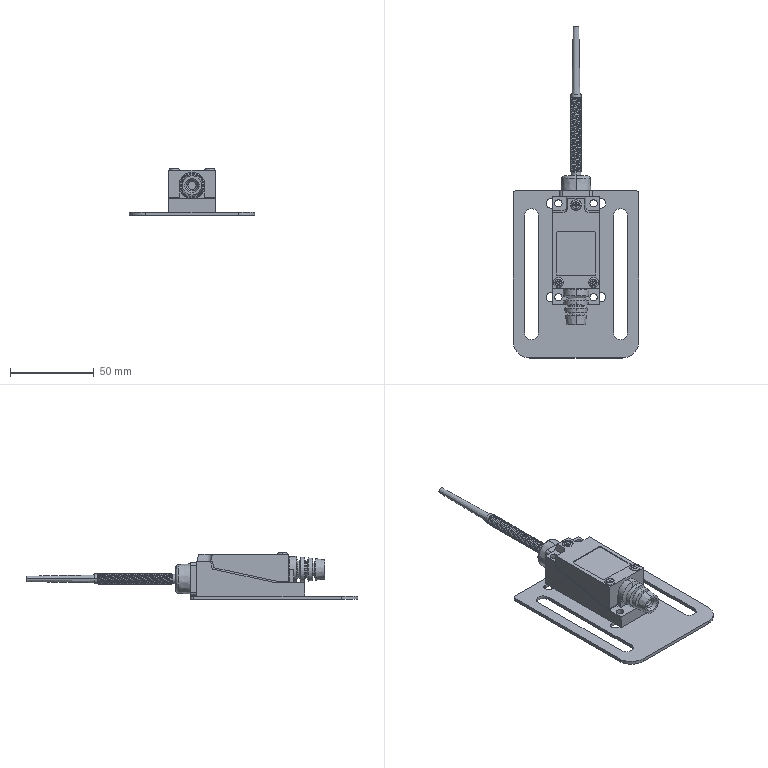Part | SolidWorks | features ICE 3, EdgeFlange 2, FlatPattern 2, SMBaseFlange 2, SheetMetal 2, BaseBody 1, Fillet 1 | 2 solids | 221 faces | box 75 x 198 x 27.9 mm | volume 57023 mm3 | plane 112 | cylinder 67 | cone 28 | spline 14 | commonest cylinder face diameters 5 x11 5.5 x10 4.3 x8 6 x6 2 x4 3 x4